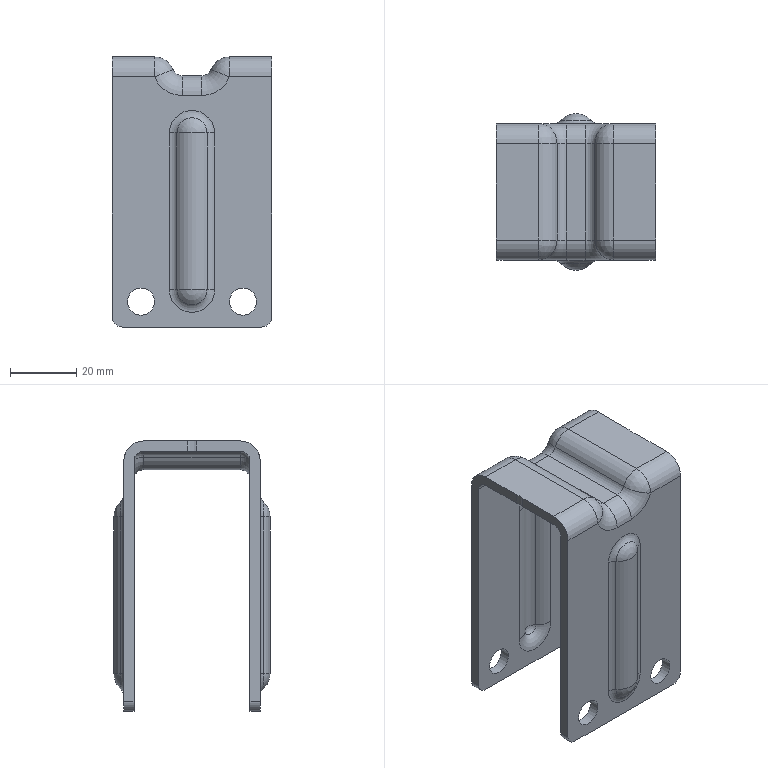Part | STEP file | PARTBODY_id358_x_t | 1 solid | 91 faces | box 48 x 47.1 x 81.415 mm | volume 28561 mm3 | cylinder 42 | sphere 17 | plane 16 | torus 16 | commonest cylinder face diameters 5.85 x10 12 x10 6.15 x6 12.3 x6 6 x4 8.17 x4